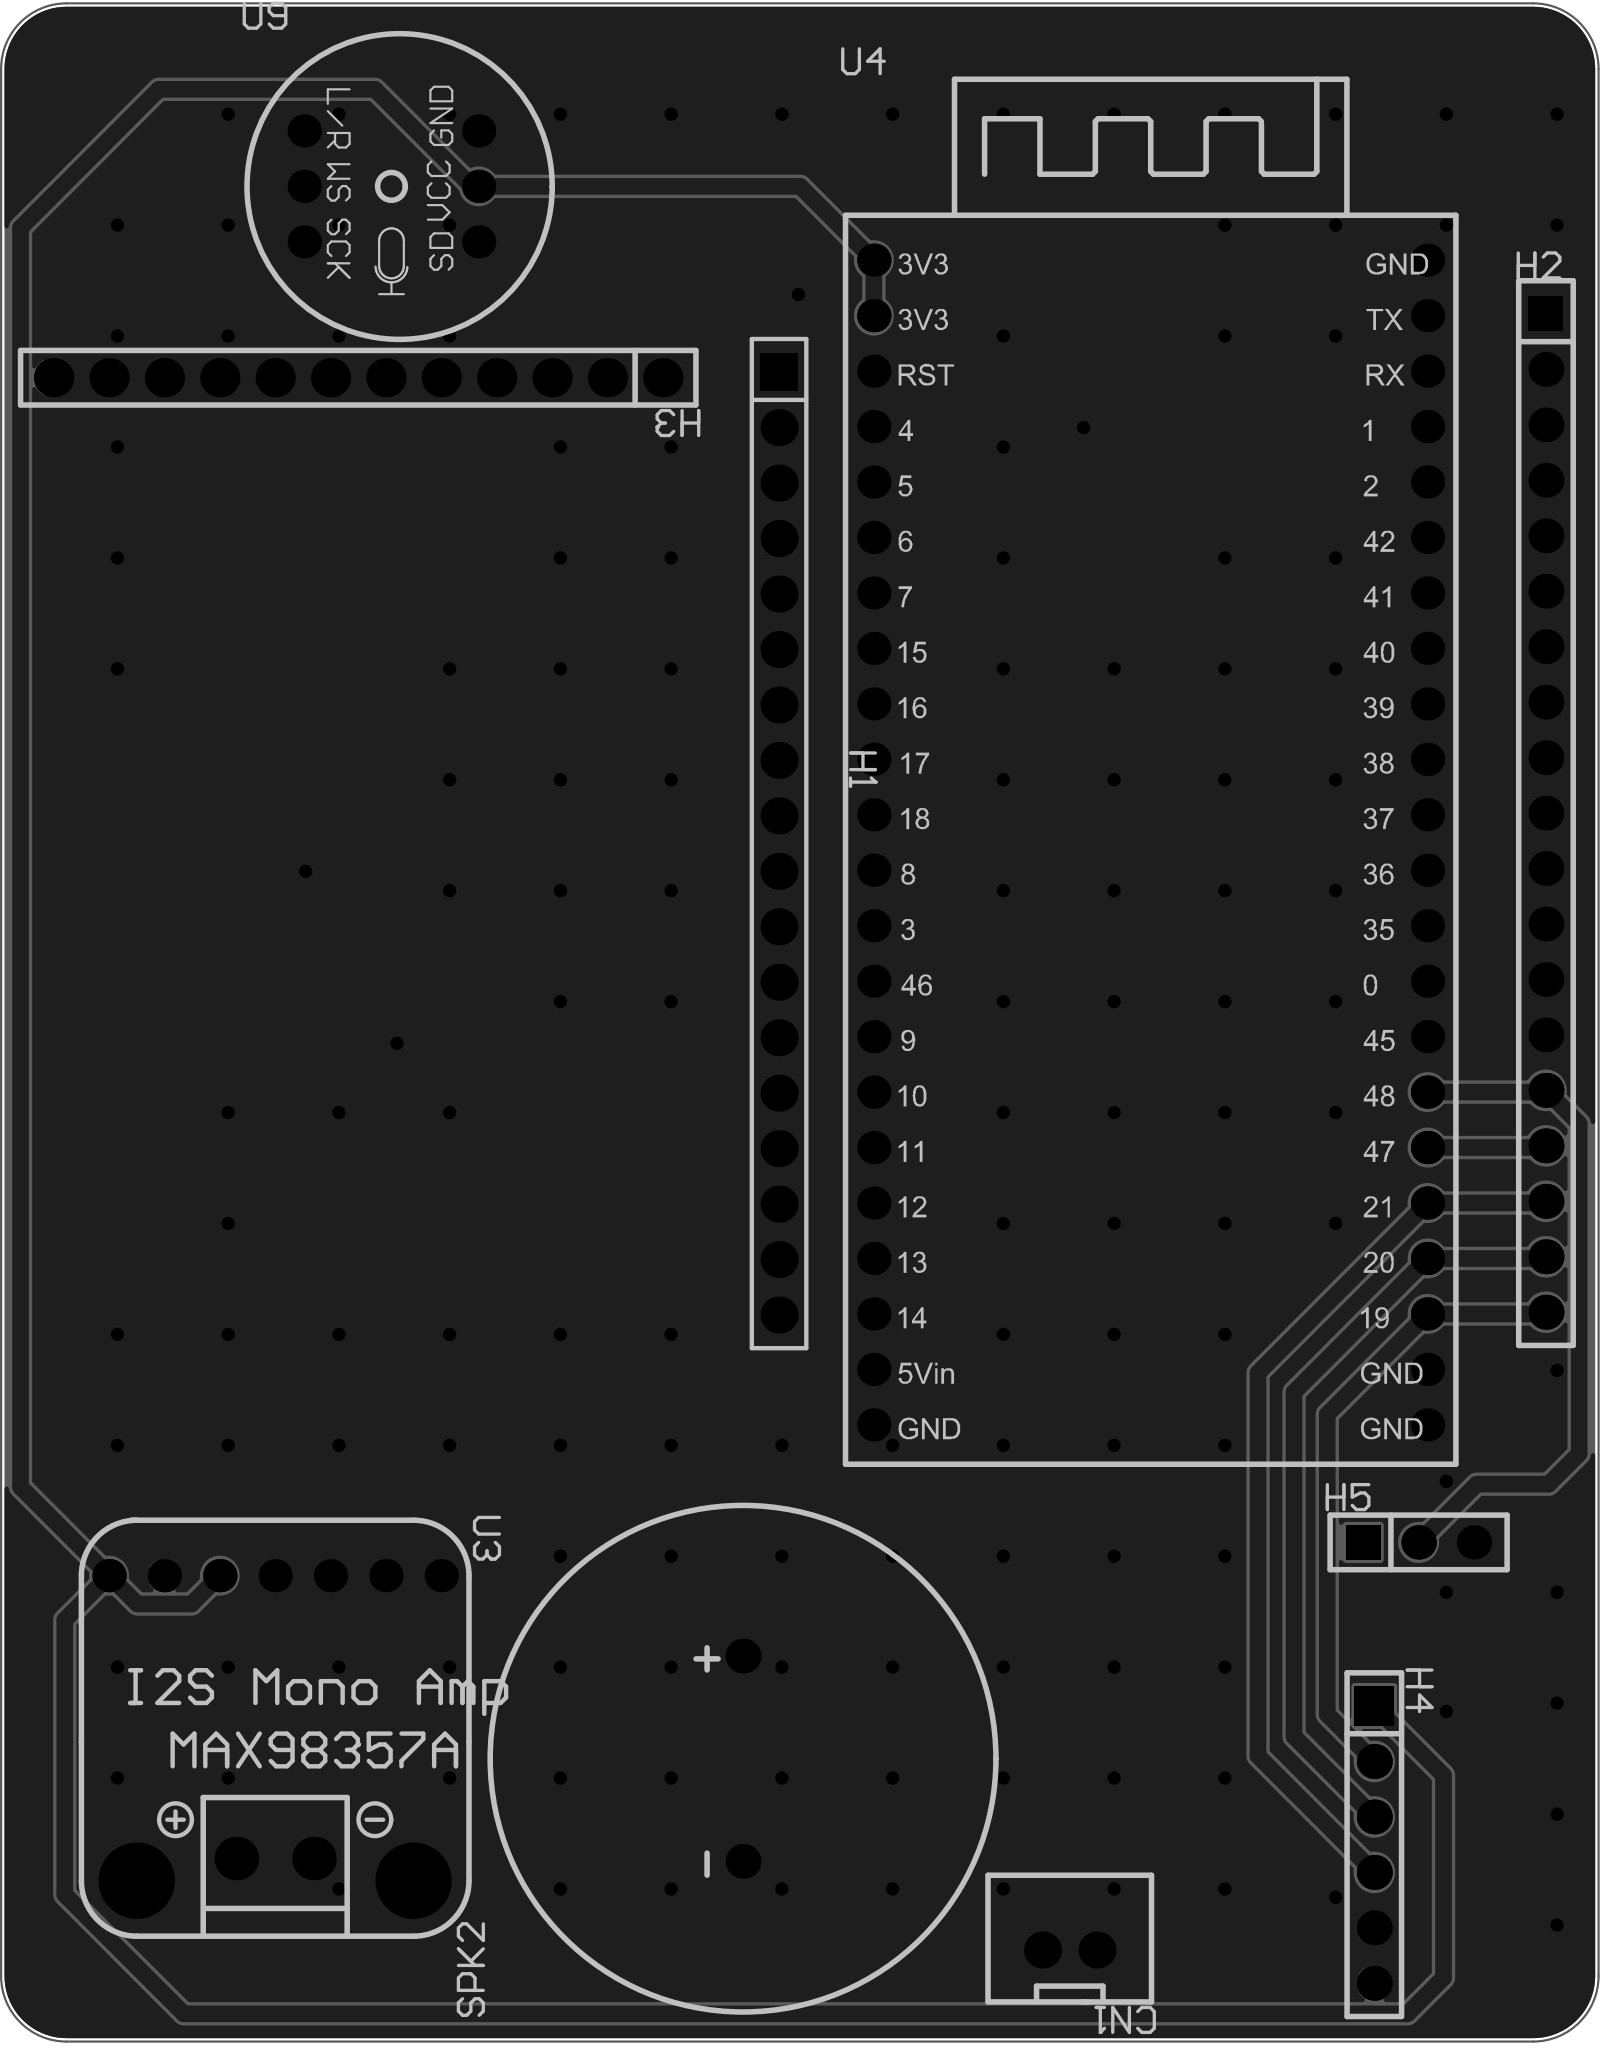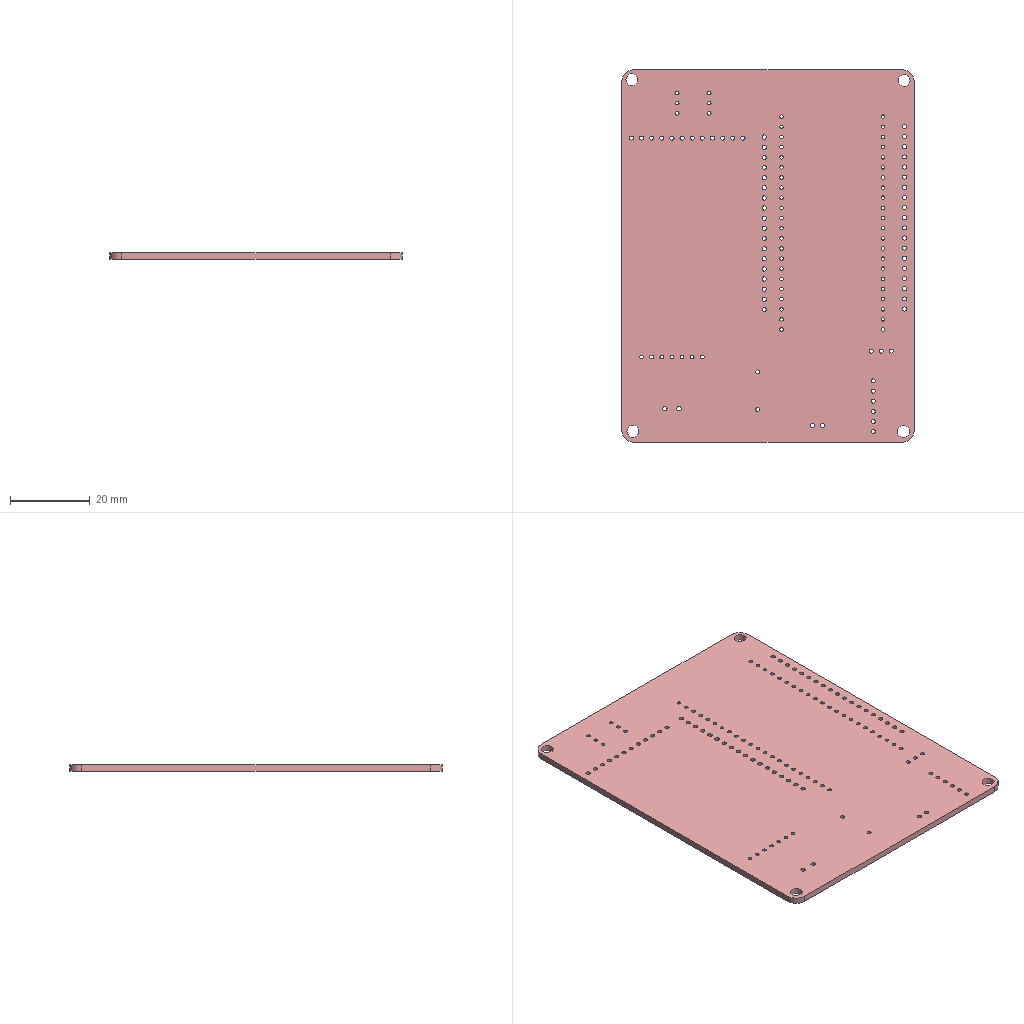Circuit board layout | Altium Designer | box 73.3 x 93.3 x 1.6 mm
Layer stack:
# Altium Designer layer stack of  (unit mm; dielectric type: 0 none, 1 core, 2 prepreg, 3 surface material)
index,name,kind,layer,copper_thickness_mm,dielectric_type,dielectric_thickness_mm,dielectric_material,dielectric_constant
0,Top Paste Mask Layer,other,,,,,,
1,Top Silkscreen Layer,other,,,,,,
2,Top Solder Mask Layer,dielectric,,,3,0.01,,3.3
3,Top Layer,copper,Top Layer,0.035,,,,
4,Dielectric1,dielectric,,,3,1.51,FR4,4.5
5,Bottom Layer,copper,Bottom Layer,0.035,,,,
6,Bottom Solder Mask Layer,dielectric,,,3,0.01,,3.3
7,Bottom Silkscreen Layer,other,,,,,,
8,Bottom Paste Mask Layer,other,,,,,,
# drill layer pairs: low layer,high layer
drill_pair,Top Layer,Bottom Layer
Part placement:
Designator,Comment,Layer,Footprint,Center-X(mm),Center-Y(mm),Rotation
SPK2,FS-2308,TopLayer,BEEP-TH_BD23.2-P9.20-D1.0,120.904,98.679,90
U3,Adafruit MAX98357 I2S Amp,TopLayer,MAX98357_I2S_AMP_MODULE,99.441,100.584,270
U4,NO,TopLayer,ESP32S3,139.603,140.638,0
U9,INMP441,TopLayer,INMP441,104.775,170.688,0
H1,,TopLayer,HDR-TH_18P-P2.54-V-F,122.555,140.589,270
H2,C2897382,TopLayer,HDR-TH_19P-P2.54-V-F,157.734,141.986,270
H3,,TopLayer,HDR-TH_12P-P2.54-V-F,103.251,161.925,180
CN1,XH2.54*2P_直插,TopLayer,CONN-TH_2P-P2.50-XH2.54-2P,135.89,89.916,180
H4,,TopLayer,HDR-TH_6P-P2.54-V-F,149.86,94.742,270
H5,,TopLayer,HDR-TH_3P-P2.54-V-F,151.892,108.585,0
Pad and via stacks:
# Altium Designer via and pad stacks of  (unit mm). Each distinct definition once, with the count of objects using it.
# via: kind,start_layer,end_layer,hole_mm,diameter_mm,mode(0 simple;1 top-mid-bottom;2 full stack),diameter_per_layer,count,example_net
# pad: kind,layer,hole_mm,hole_type(0 round;1 square;2 slot),plating,top_size,top_shape(1 round;2 rect;3 octagon;9 rounded rect),mid_size,bottom_size,mode,footprint,size_per_layer,count,example
pad,Multi-Layer,1,0,plated,1.6x1.6,1,1.6x1.6,1.6x1.6,0,BEEP-TH_BD23.2-P9.20-D1.0,,2,SPK2.1
pad,Multi-Layer,0.9144,0,plated,1.524x1.524,1,1.524x1.524,1.524x1.524,0,MAX98357 I2S AMP MODULE,,7,U3.1
pad,Multi-Layer,1.1,0,plated,2x2,1,2x2,2x2,0,MAX98357 I2S AMP MODULE,,2,U3.9
pad,Multi-Layer,0.9144,0,plated,1.524x1.524,1,1.524x1.524,1.524x1.524,0,ESP32S3,,44,U4.1
pad,Multi-Layer,0.9144,0,plated,1.524x1.524,1,1.524x1.524,1.524x1.524,0,INMP441,,6,U9.5
pad,Multi-Layer,1.1,0,plated,1.7x1.7,2,1.7x1.7,1.7x1.7,0,HDR-TH_18P-P2.54-V-F,,1,H1.1
pad,Multi-Layer,1.1,0,plated,1.7x1.7,1,1.7x1.7,1.7x1.7,0,HDR-TH_18P-P2.54-V-F,,17,H1.2
pad,Multi-Layer,1.05,0,plated,1.6x1.6,1,1.6x1.6,1.6x1.6,0,HDR-TH_19P-P2.54-V-F,,18,H2.19
pad,Multi-Layer,1.05,0,plated,1.6x1.6,2,1.6x1.6,1.6x1.6,0,HDR-TH_19P-P2.54-V-F,,1,H2.1
pad,Multi-Layer,1.05,0,plated,1.8x1.8,1,1.8x1.8,1.8x1.8,0,HDR-TH_12P-P2.54-V-F,,12,H3.1
pad,Multi-Layer,1.05,0,plated,1.7x1.7,1,1.7x1.7,1.7x1.7,0,CONN-TH_2P-P2.50-XH2.54-2P,,2,CN1.2
pad,Multi-Layer,1.02,0,plated,1.6x1.6,1,1.6x1.6,1.6x1.6,0,HDR-TH_6P-P2.54-V-F,,5,H4.6
pad,Multi-Layer,1.02,0,plated,1.8x1.8,2,1.8x1.8,1.8x1.8,0,HDR-TH_6P-P2.54-V-F,,1,H4.1
pad,Multi-Layer,1.02,0,plated,1.575x1.575,1,1.575x1.575,1.575x1.575,0,HDR-TH_3P-P2.54-V-F,,2,H5.3
pad,Multi-Layer,1.02,0,plated,1.575x1.575,2,1.575x1.575,1.575x1.575,0,HDR-TH_3P-P2.54-V-F,,1,H5.1
via,Top Layer,Bottom Layer,2.499,3.5,0,,2,
via,Top Layer,Bottom Layer,0.3048,0.61,0,,4,9
via,Top Layer,Bottom Layer,0.3048,0.6096,0,,143,GND
Copper pours:
name,layer,net,type(0 solid;1 hatched;2 none)
Top Layer-GND,Top Layer,GND,0
Bottom Layer-GND,Bottom Layer,GND,0
Design rules, without the lines most boards share:
# Altium Designer design rules of  (exported by Altium Designer, unit mm)
# columns: name | kind | enabled | priority | scope1 | scope2 | descriptor | typed fields (field=value)
Plane_Default | 0 | disabled | 1 | All | All | Clearance Constraint (Gap=6mil) (Disabled)(All),(All) | gap=0.1524
Plane_Default_1 | 63 | disabled | 1 | All | All | Board Clearance Constraint (Gap=0mil) (Disabled)(All) |
Copper_Default | 0 | disabled | 2 | All | All | Clearance Constraint (Gap=6mil) (Disabled)(All),(All) | gap=0.1524
Copper_Default_1 | 63 | disabled | 2 | All | All | Board Clearance Constraint (Gap=0mil) (Disabled)(All) |
Copper_gge24019 | 0 | disabled | 3 | All | All | Clearance Constraint (Gap=6mil) (Disabled)(All),(All) | gap=0.1524
Copper_gge24019_1 | 63 | disabled | 3 | All | All | Board Clearance Constraint (Gap=0mil) (Disabled)(All) |
Default | 0 | enabled | 4 | All | All | Clearance Constraint (Gap=6mil) (All),(All) | gap=0.1524
Default_1 | 63 | enabled | 4 | All | All | Board Clearance Constraint (Gap=0mil) (All) |
otherClearance | 52 | enabled | 1 | All | All | Hole To Hole Clearance (Gap=11.8mil) (All),(All) | gap=0.2997
Default_2 | 2 | enabled | 1 | All | All | Width Constraint (Min=10mil) (Max=1000mil) (Preferred=30mil) (All) |
Default_3 | 11 | enabled | 1 | All | All | Routing Via (MinHoleWidth=12mil) (MaxHoleWidth=2362mil) (PreferredHoleWidth=12mil) (MinWidth=24mil) (MaxWidth=3938mil) (PreferedWidth=24mil) (All) | via_min_hole=0.3048 via_max_hole=59.995 via_preferred_diameter=0.6096 via_preferred_hole=0.3048
Default_4 | 6 | enabled | 1 | All | All | Power Plane Connect Rule(Relief Connect )(Expansion=20mil) (Conductor Width=0mil) (Air Gap=10mil) (Entries=4) (All) | relief_conductor_width=0 relief_entries=4 relief_expansion=0.508
gge24019 | 20 | disabled | 1 | All | All | Polygon Connect Rule(Relief Connect )(Conductor Width=0mil) (Relief Angle=90 Angle) (Entries=4) (Air Gap Width=1mil) (Disabled)(All),(All) | connect_style(0=relief,1=direct,2=none)=0 relief_conductor_width=0 relief_entries=4
Default_5 | 20 | enabled | 2 | All | All | Polygon Connect Rule(Relief Connect )(Conductor Width=0mil) (Relief Angle=90 Angle) (Entries=4) (Air Gap Width=1mil) (All),(All) | connect_style(0=relief,1=direct,2=none)=0 relief_conductor_width=0 relief_entries=4
Common | 14 | enabled | 1 | All | All | Paste Mask Expansion (Expansion =0mil) (All) | expansion=0
Common_1 | 13 | enabled | 2 | All | All | Solder Mask Expansion (Expansion =2mil) (All) | expansion=0.0508
Common_2 | 13 | enabled | 1 | IsVia | All | Solder Mask Expansion (Expansion =-1000mil) (IsVia) | expansion=-25.4